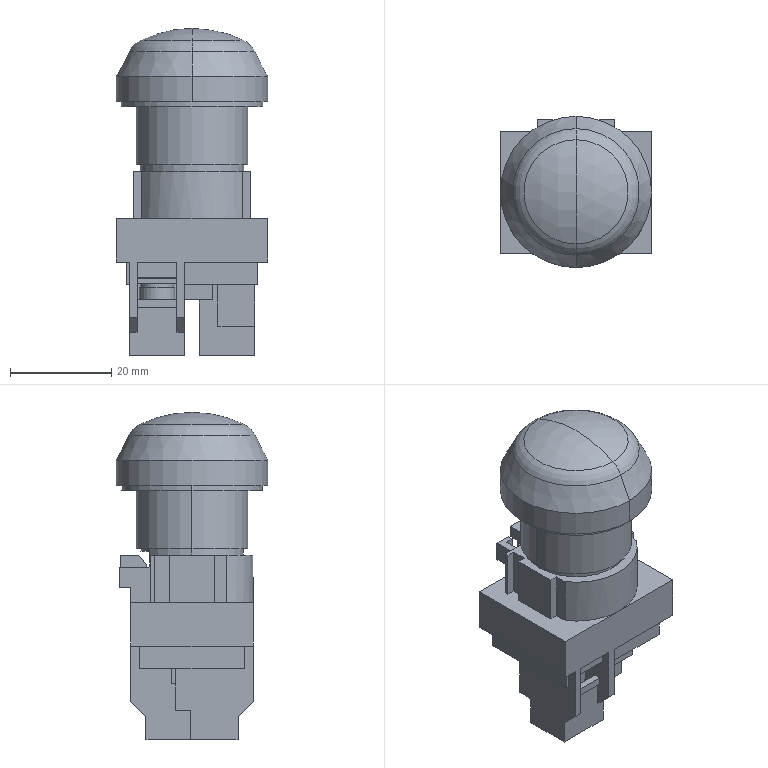Part | STEP file | M22N-BG-TGA-GC | 1 solid | 156 faces | box 30 x 29.9 x 64.7 mm | volume 28524 mm3 | plane 129 | cylinder 21 | torus 2 | sphere 2 | cone 2 | commonest cylinder face diameters 6.4 x4 6.6 x4 7 x4 20.4 x2 22 x2 28 x2